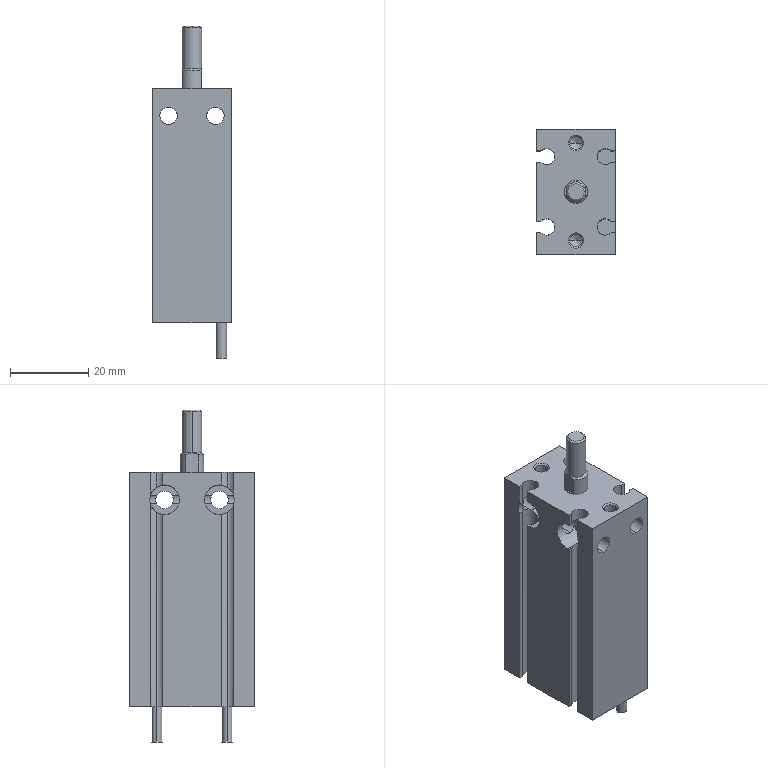Part | STEP file | CDU16-20D-A93 (0) | 1 solid | 155 faces | box 20 x 32 x 85 mm | volume 33757 mm3 | cylinder 72 | plane 55 | cone 28 | commonest cylinder face diameters 7.6 x24 4.5 x16 3.242 x8 4.2 x8 2.7 x4 4 x4